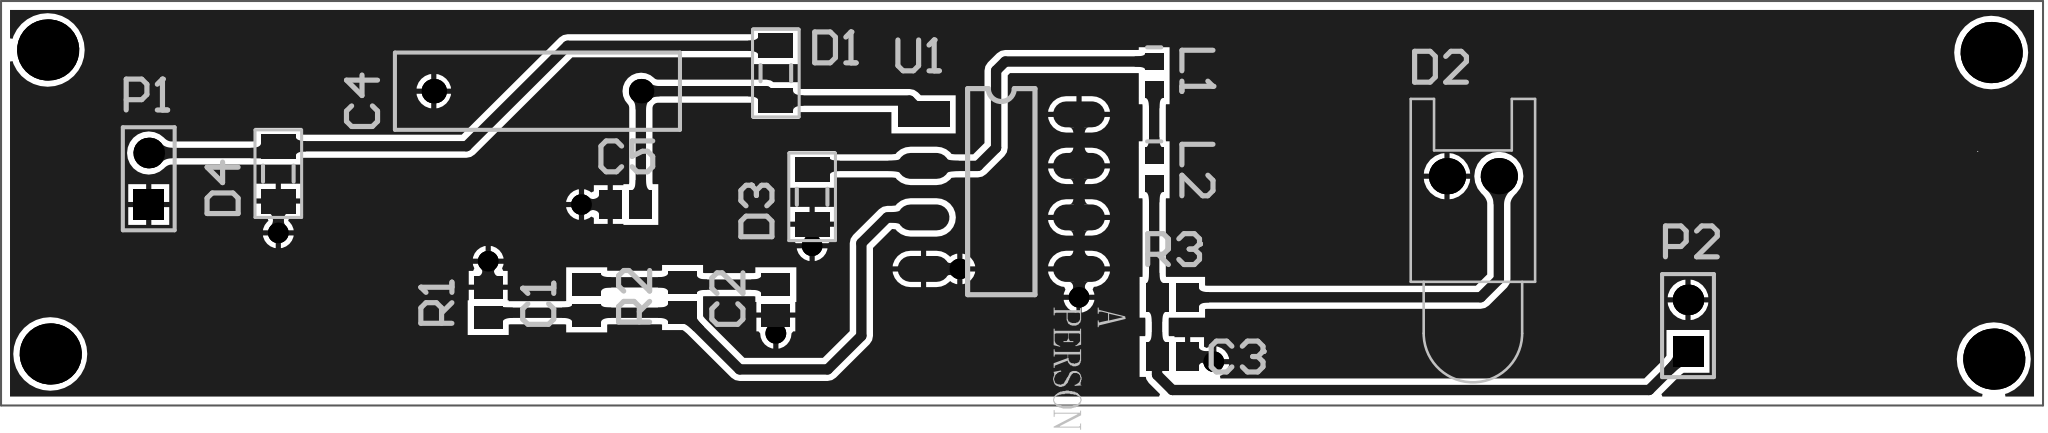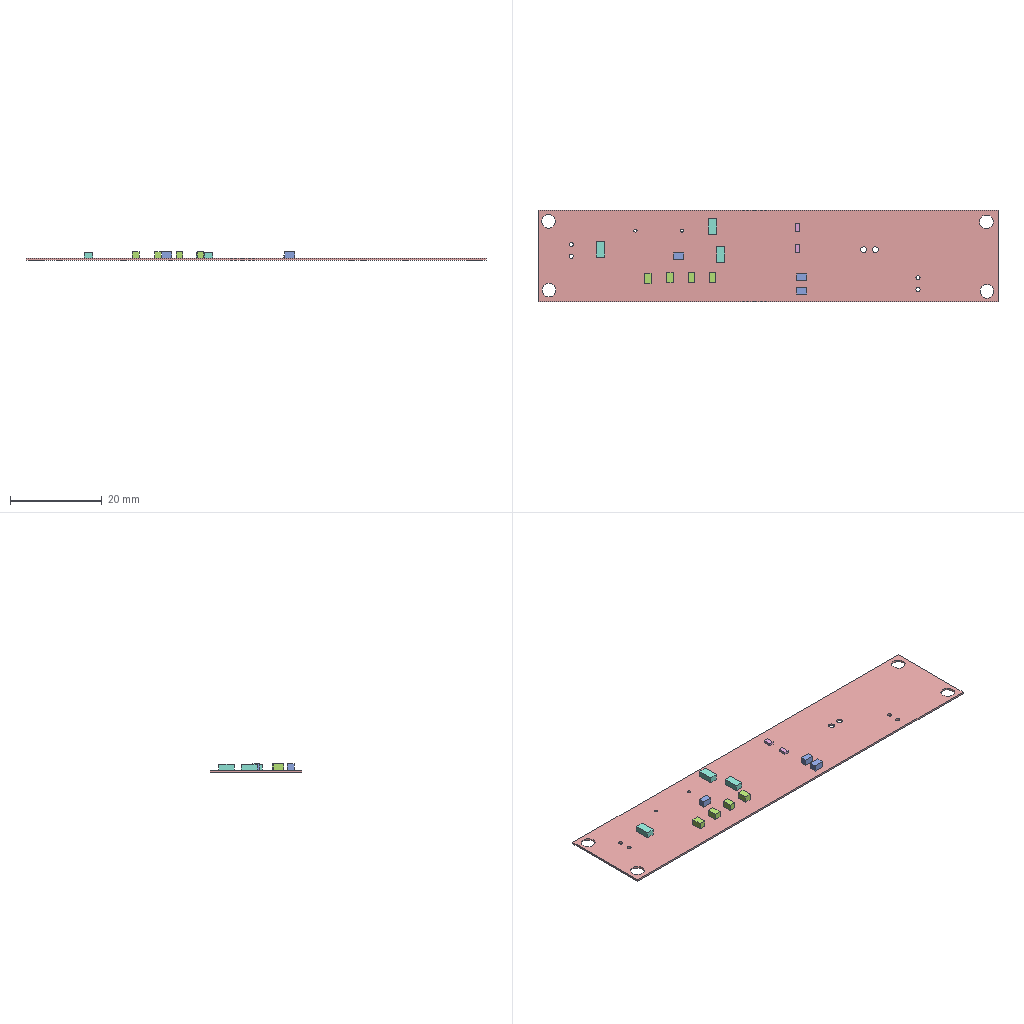Circuit board layout | Altium Designer | box 100.1 x 19.9 x 1.8 mm
Layer stack:
# Altium Designer layer stack of  (unit mm; dielectric type: 0 none, 1 core, 2 prepreg, 3 surface material)
index,name,kind,layer,copper_thickness_mm,dielectric_type,dielectric_thickness_mm,dielectric_material,dielectric_constant
0,Top Paste,other,,,,,,
1,Top Overlay,other,,,,,,
2,Top Solder,dielectric,,,3,0.0102,Solder Resist,3.5
3,Top Layer,copper,Top Layer,0.0356,,,,
4,Dielectric 1,dielectric,,,0,0.32,FR-4,4.8
5,Bottom Layer,copper,Bottom Layer,0.0356,,,,
6,Bottom Solder,dielectric,,,3,0.0102,Solder Resist,3.5
7,Bottom Overlay,other,,,,,,
8,Bottom Paste,other,,,,,,
# drill layer pairs: low layer,high layer
drill_pair,Top Layer,Bottom Layer
Part placement:
Designator,Comment,Layer,Footprint,Center-X(mm),Center-Y(mm),Rotation
U1,XL1509,TopLayer,ESOP8,74.422,35.941,0
R3,Res2,TopLayer,C0805,82.804,30.734,0
R2,6.8K,TopLayer,C0805,58.801,30.722,90
R1,2.2K,TopLayer,C0805,49.276,30.48,270
P2,Header 2,TopLayer,HDR1X2,108.077,29.337,90
P1,Header 2,TopLayer,HDR1X2,32.639,36.576,90
L2,Inductor,TopLayer,INDC1608L,81.915,37.019,270
L1,68UH,TopLayer,INDC1608L,81.915,41.656,270
D4,SMBJ48CA,TopLayer,C1206,38.989,36.83,90
D3,SS36F,TopLayer,C1206,65.151,35.687,90
D2,LED0,TopLayer,LED-0,97.536,36.703,0
D1,SS36F,TopLayer,C1206,63.373,41.783,270
C5,1UF,TopLayer,C0805,56.007,35.306,0
C4,220UF,TopLayer,RAD-0.4,51.689,40.894,180
C3,220UF,TopLayer,C0805,82.804,27.813,180
C2,220UF,TopLayer,C0805,63.373,30.607,90
C1,6.6UF,TopLayer,C0805,54.102,30.607,90
Pad and via stacks:
# Altium Designer via and pad stacks of  (unit mm). Each distinct definition once, with the count of objects using it.
# via: kind,start_layer,end_layer,hole_mm,diameter_mm,mode(0 simple;1 top-mid-bottom;2 full stack),diameter_per_layer,count,example_net
# pad: kind,layer,hole_mm,hole_type(0 round;1 square;2 slot),plating,top_size,top_shape(1 round;2 rect;3 octagon;9 rounded rect),mid_size,bottom_size,mode,footprint,size_per_layer,count,example
pad,Top Layer,0,0,plated,1.4x1.1,2,1.4x1.1,1.4x1.1,0,C0805,,14,C1.2
pad,Top Layer,0,0,plated,2.54x1.27,2,2.54x1.27,2.54x1.27,0,ESOP8,,1,U1.1
pad,Top Layer,0,0,plated,2.54x1.27,1,2.54x1.27,2.54x1.27,0,ESOP8,,7,U1.2
pad,Top Layer,0,0,plated,1.7x1.2,2,1.7x1.2,1.7x1.2,0,C1206,,6,D1.1
pad,Top Layer,0,0,plated,0.9x0.8,2,0.9x0.8,0.9x0.8,0,INDC1608L,,4,L2.2
pad,Multi-Layer,3,0,plated,3x3,1,3x3,3x3,0,,,4,3
pad,Multi-Layer,1.27,0,plated,1.778x1.778,1,1.778x1.778,1.778x1.778,0,LED-0,,2,D2.1
pad,Multi-Layer,0.7,0,plated,1.2x1.2,1,1.2x1.2,1.2x1.2,0,RAD-0.4,,2,C4.1
pad,Multi-Layer,0.9,0,plated,1.5x1.5,2,1.5x1.5,1.5x1.5,0,HDR1X2,,2,P2.1
pad,Multi-Layer,0.9,0,plated,1.5x1.5,1,1.5x1.5,1.5x1.5,0,HDR1X2,,2,P2.2
via,Top Layer,Bottom Layer,0.635,1.016,0,,8,GND
Copper pours:
name,layer,net,type(0 solid;1 hatched;2 none)
D,Top Layer,GND,0
Design rules, without the lines most boards share:
# Altium Designer design rules of  (exported by Altium Designer, unit mm)
# columns: name | kind | enabled | priority | scope1 | scope2 | descriptor | typed fields (field=value)
SilkToSilkClearance | 55 | enabled | 1 | All | All | Silk to Silk (Clearance=0mil) (All),(All) |
SilkToSolderMaskClearance | 54 | enabled | 1 | IsPad | All | Silk To Solder Mask (Clearance=0mil) (IsPad),(All) |
MinimumSolderMaskSliver | 53 | enabled | 1 | All | All | Minimum Solder Mask Sliver (Gap=0mil) (All),(All) |
HoleToHoleClearance | 52 | enabled | 1 | All | All | Hole To Hole Clearance (Gap=10mil) (All),(All) | gap=0.254
DiffPairsRouting | 51 | enabled | 1 | All | All | Differential Pairs Uncoupled Length using the Gap Constraints (Min=10mil) (Max=10mil) (Prefered=10mil)  and Width Constraints (Min=15mil) (Max=15mil) (Prefered=15mil) (All) |
SolderMaskExpansion | 13 | enabled | 1 | All | All | Solder Mask Expansion (Expansion =4mil) (All) | expansion=0.1016
PasteMaskExpansion | 14 | enabled | 1 | All | All | Paste Mask Expansion (Expansion =0mil) (All) | expansion=0
RoutingVias | 11 | enabled | 1 | All | All | Routing Via (MinHoleWidth=28mil) (MaxHoleWidth=28mil) (PreferredHoleWidth=28mil) (MinWidth=50mil) (MaxWidth=50mil) (PreferedWidth=50mil) (All) | via_min_hole=0.7112 via_max_hole=0.7112 via_preferred_diameter=1.27 via_preferred_hole=0.7112
Width | 2 | enabled | 1 | All | All | Width Constraint (Min=10mil) (Max=39.37mil) (Preferred=10mil) (All) |
PolygonConnect | 20 | enabled | 1 | All | All | Polygon Connect Rule(Relief Connect )(Conductor Width=10mil) (Relief Angle=90 Angle) (Entries=4) (Air Gap Width=10mil) (All),(All) | connect_style(0=relief,1=direct,2=none)=0 relief_conductor_width=0.254 relief_entries=4
PlaneConnect | 6 | enabled | 1 | All | All | Power Plane Connect Rule(Relief Connect )(Expansion=20mil) (Conductor Width=10mil) (Air Gap=10mil) (Entries=4) (All) | relief_conductor_width=0.254 relief_entries=4 relief_expansion=0.508
Clearance | 0 | enabled | 1 | All | All | Clearance Constraint (Gap=12mil) (All),(All) | gap=0.3048